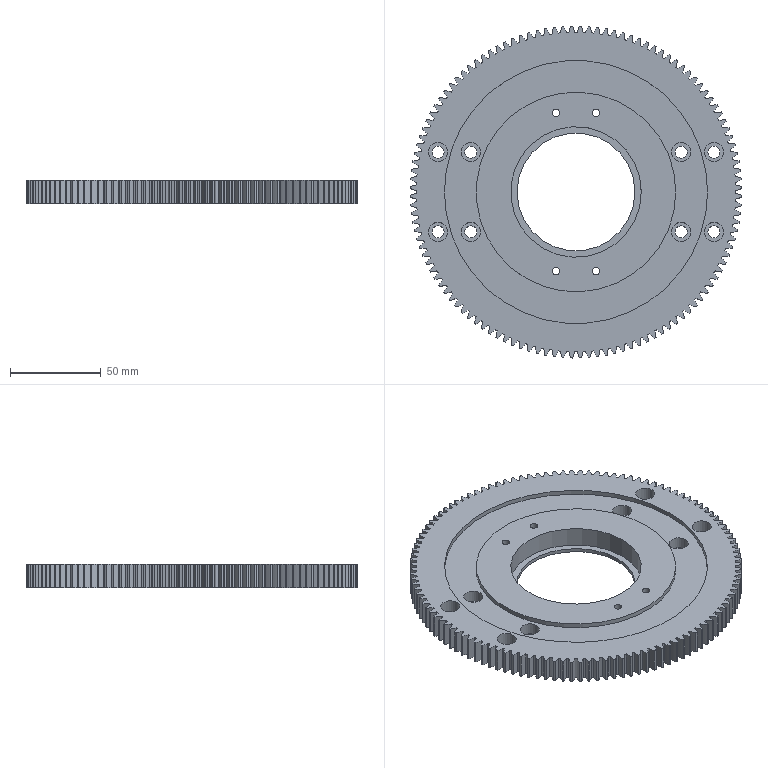Part | NX | features BREP 1 | 1 solid | 517 faces | box 182.961 x 182.961 x 13 mm | volume 252915 mm3 | cylinder 504 | plane 13 | commonest cylinder face diameters 72 x241 176.248 x120 183 x120 6.6 x8 10.5 x8 4.2 x4